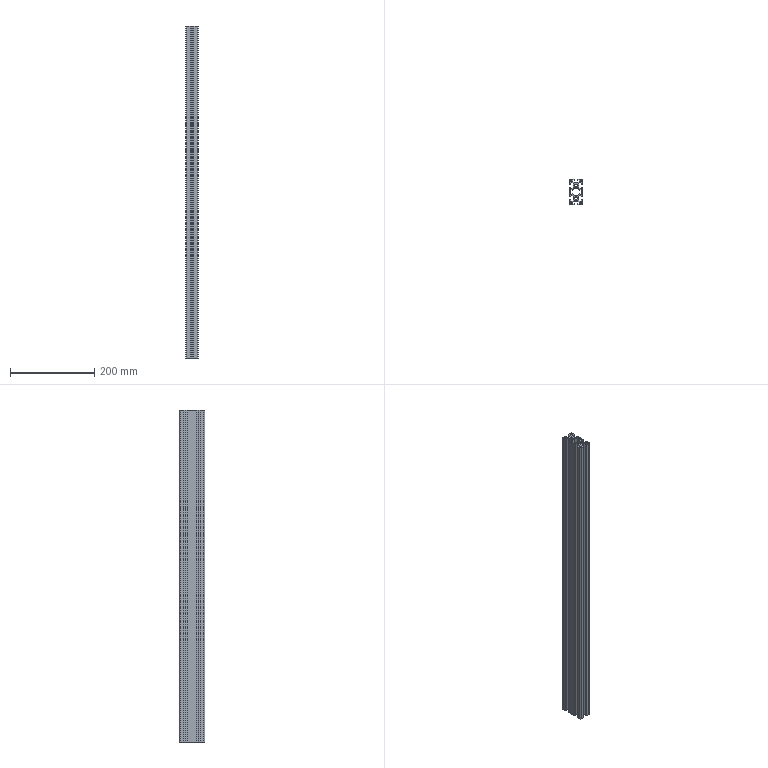Part | STEP file | Guide wheel mechanism revised.sldasm-Part-437 | 1 solid | 136 faces | box 30 x 60 x 788 mm | volume 468506 mm3 | plane 94 | cylinder 38 | cone 4 | commonest cylinder face diameters 0.6 x16 4.2 x8 2 x4 4 x4 6.647 x4 12 x2